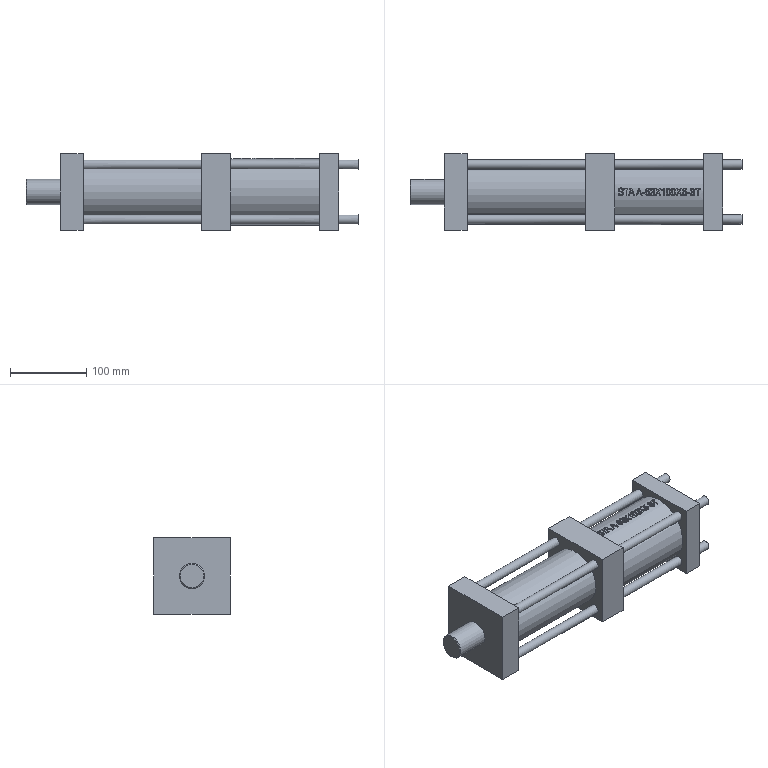Part | STEP file | Tube feed_id746_x_t | 1 solid | 172 faces | box 435 x 100 x 100 mm | volume 2482433 mm3 | plane 73 | spline 62 | cylinder 36 | cone 1 | commonest cylinder face diameters 89 x16 12 x12 87 x6 33 x1 75 x1